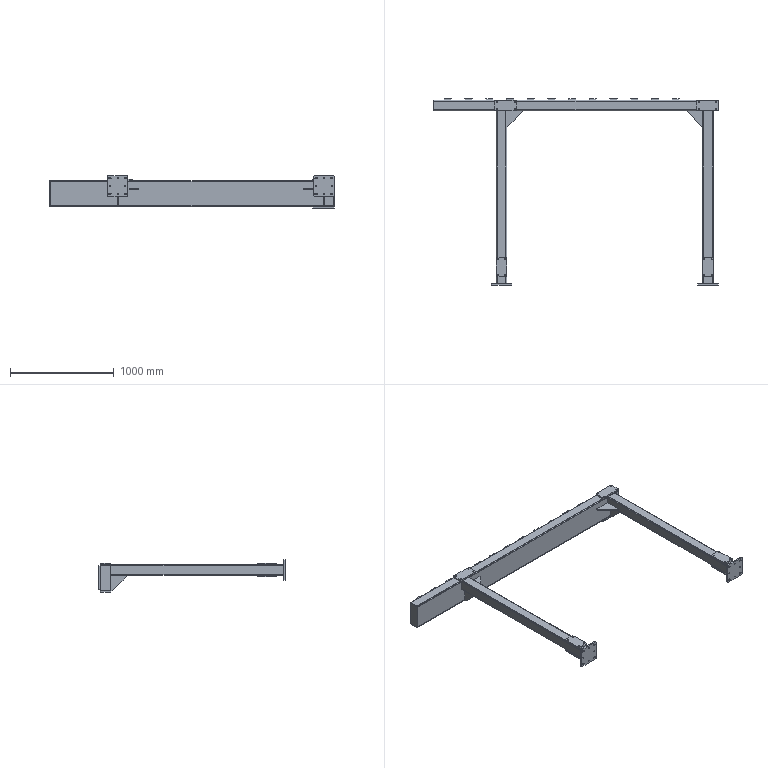Part | SolidWorks | features ICE 8, HoleWzd 5, MirrorSolid 4, WeldMemberFeat 2, LPattern 1, WeldCornerFeat 1, WeldmentFeature 1 | 30 solids | 536 faces | box 2745 x 1798 x 315 mm | volume 19263192 mm3 | plane 296 | cylinder 192 | cone 48 | commonest cylinder face diameters 10.2 x96 5 x48 8 x20 13.5 x16 16 x12